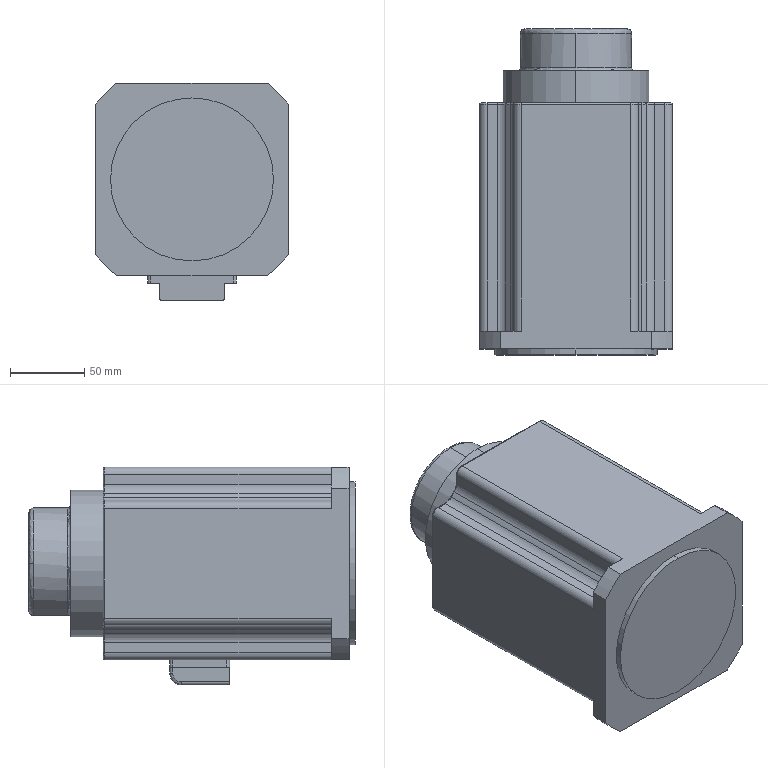Part | STEP file | Link1_mot | 1 solid | 116 faces | box 130 x 220 x 147 mm | volume 2850182 mm3 | cylinder 55 | plane 31 | spline 27 | torus 3 | commonest cylinder face diameters 2 x14 4 x9 16 x9 10 x8 130 x4 165 x4